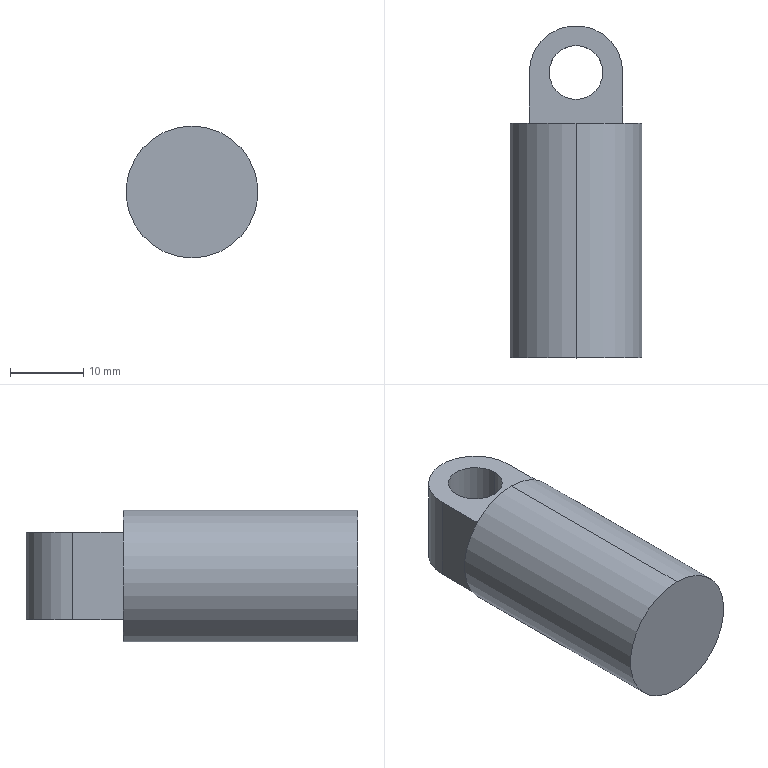Part | SolidWorks | features Cut 1, Extrusion 1, ICE 1 | 1 solid | 11 faces | box 18 x 45.316 x 18 mm | volume 9465 mm3 | plane 6 | cylinder 5 | commonest cylinder face diameters 7.349 x2 18 x2 12.778 x1
STEP:
#1=CARTESIAN_POINT('',(-30.863,-16.288,16.608));
#2=VERTEX_POINT('',#1);
#3=CARTESIAN_POINT('',(-23.514,-16.288,16.608));
#4=VERTEX_POINT('',#3);
#5=CARTESIAN_POINT('',(-27.189,-16.288,16.608));
#6=DIRECTION('',(0.,0.,1.));
#7=DIRECTION('',(-1.,0.,0.));
#8=AXIS2_PLACEMENT_3D('',#5,#6,#7);
#9=CIRCLE('',#8,3.675);
#10=EDGE_CURVE('',#2,#4,#9,.T.);
#11=ORIENTED_EDGE('',*,*,#10,.T.);
#12=CARTESIAN_POINT('',(-23.514,-16.288,4.608));
#13=VERTEX_POINT('',#12);
#14=CARTESIAN_POINT('',(-23.514,-16.288,27.001));
#15=DIRECTION('',(0.,0.,-1.));
#16=VECTOR('',#15,1000.);
#17=LINE('',#14,#16);
#18=EDGE_CURVE('',#4,#13,#17,.T.);
#19=ORIENTED_EDGE('',*,*,#18,.T.);
#20=CARTESIAN_POINT('',(-30.863,-16.288,4.608));
#21=VERTEX_POINT('',#20);
#22=CARTESIAN_POINT('',(-27.189,-16.288,4.608));
#23=DIRECTION('',(0.,0.,-1.));
#24=DIRECTION('',(-1.,0.,0.));
#25=AXIS2_PLACEMENT_3D('',#22,#23,#24);
#26=CIRCLE('',#25,3.675);
#27=EDGE_CURVE('',#13,#21,#26,.T.);
#28=ORIENTED_EDGE('',*,*,#27,.T.);
#29=CARTESIAN_POINT('',(-30.863,-16.288,27.001));
#30=DIRECTION('',(0.,0.,-1.));
#31=VECTOR('',#30,1000.);
#32=LINE('',#29,#31);
#33=EDGE_CURVE('',#2,#21,#32,.T.);
#34=ORIENTED_EDGE('',*,*,#33,.F.);
#35=EDGE_LOOP('',(#11,#19,#28,#34));
#36=FACE_OUTER_BOUND('',#35,.T.);
#37=CARTESIAN_POINT('',(-27.189,-16.288,27.001));
#38=DIRECTION('',(0.,0.,-1.));
#39=DIRECTION('',(-1.,0.,0.));
#40=AXIS2_PLACEMENT_3D('',#37,#38,#39);
#41=CYLINDRICAL_SURFACE('',#40,3.675);
#42=ADVANCED_FACE('',(#36),#41,.F.);
#43=CARTESIAN_POINT('',(-27.189,-55.215,1.608));
#44=VERTEX_POINT('',#43);
#45=CARTESIAN_POINT('',(-27.189,-55.215,19.608));
#46=VERTEX_POINT('',#45);
#47=CARTESIAN_POINT('',(-27.189,-55.215,10.608));
#48=DIRECTION('',(0.,-1.,0.));
#49=DIRECTION('',(0.,0.,-1.));
#50=AXIS2_PLACEMENT_3D('',#47,#48,#49);
#51=CIRCLE('',#50,9.);
#52=EDGE_CURVE('',#44,#46,#51,.T.);
#53=ORIENTED_EDGE('',*,*,#52,.F.);
#54=CARTESIAN_POINT('',(-27.189,-23.215,1.608));
#55=VERTEX_POINT('',#54);
#56=CARTESIAN_POINT('',(-27.189,-55.215,1.608));
#57=DIRECTION('',(0.,1.,0.));
#58=VECTOR('',#57,1000.);
#59=LINE('',#56,#58);
#60=EDGE_CURVE('',#44,#55,#59,.T.);
#61=ORIENTED_EDGE('',*,*,#60,.T.);
#62=CARTESIAN_POINT('',(-27.189,-23.215,19.608));
#63=VERTEX_POINT('',#62);
#64=CARTESIAN_POINT('',(-27.189,-23.215,10.608));
#65=DIRECTION('',(0.,-1.,0.));
#66=DIRECTION('',(0.,0.,-1.));
#67=AXIS2_PLACEMENT_3D('',#64,#65,#66);
#68=CIRCLE('',#67,9.);
#69=EDGE_CURVE('',#55,#63,#68,.T.);
#70=ORIENTED_EDGE('',*,*,#69,.T.);
#71=CARTESIAN_POINT('',(-27.189,-55.215,19.608));
#72=DIRECTION('',(0.,1.,0.));
#73=VECTOR('',#72,1000.);
#74=LINE('',#71,#73);
#75=EDGE_CURVE('',#46,#63,#74,.T.);
#76=ORIENTED_EDGE('',*,*,#75,.F.);
#77=EDGE_LOOP('',(#53,#61,#70,#76));
#78=FACE_OUTER_BOUND('',#77,.T.);
#79=CARTESIAN_POINT('',(-27.189,-55.215,10.608));
#80=DIRECTION('',(0.,1.,0.));
#81=DIRECTION('',(0.,0.,1.));
#82=AXIS2_PLACEMENT_3D('',#79,#80,#81);
#83=CYLINDRICAL_SURFACE('',#82,9.);
#84=ADVANCED_FACE('',(#78),#83,.T.);
#85=CARTESIAN_POINT('',(-33.578,-16.288,16.608));
#86=VERTEX_POINT('',#85);
#87=CARTESIAN_POINT('',(-20.8,-16.288,16.608));
#88=VERTEX_POINT('',#87);
#89=CARTESIAN_POINT('',(-27.189,-16.288,16.608));
#90=DIRECTION('',(0.,0.,-1.));
#91=DIRECTION('',(-1.,0.,0.));
#92=AXIS2_PLACEMENT_3D('',#89,#90,#91);
#93=CIRCLE('',#92,6.389);
#94=EDGE_CURVE('',#86,#88,#93,.T.);
#95=ORIENTED_EDGE('',*,*,#94,.T.);
#96=CARTESIAN_POINT('',(-20.8,-16.288,4.608));
#97=VERTEX_POINT('',#96);
#98=CARTESIAN_POINT('',(-20.8,-16.288,4.608));
#99=DIRECTION('',(0.,0.,1.));
#100=VECTOR('',#99,1000.);
#101=LINE('',#98,#100);
#102=EDGE_CURVE('',#97,#88,#101,.T.);
#103=ORIENTED_EDGE('',*,*,#102,.F.);
#104=CARTESIAN_POINT('',(-33.578,-16.288,4.608));
#105=VERTEX_POINT('',#104);
#106=CARTESIAN_POINT('',(-27.189,-16.288,4.608));
#107=DIRECTION('',(0.,0.,-1.));
#108=DIRECTION('',(-1.,0.,0.));
#109=AXIS2_PLACEMENT_3D('',#106,#107,#108);
#110=CIRCLE('',#109,6.389);
#111=EDGE_CURVE('',#105,#97,#110,.T.);
#112=ORIENTED_EDGE('',*,*,#111,.F.);
#113=CARTESIAN_POINT('',(-33.578,-16.288,4.608));
#114=DIRECTION('',(0.,0.,1.));
#115=VECTOR('',#114,1000.);
#116=LINE('',#113,#115);
#117=EDGE_CURVE('',#105,#86,#116,.T.);
#118=ORIENTED_EDGE('',*,*,#117,.T.);
#119=EDGE_LOOP('',(#95,#103,#112,#118));
#120=FACE_OUTER_BOUND('',#119,.T.);
#121=CARTESIAN_POINT('',(-27.189,-16.288,4.608));
#122=DIRECTION('',(0.,0.,1.));
#123=DIRECTION('',(1.,0.,0.));
#124=AXIS2_PLACEMENT_3D('',#121,#122,#123);
#125=CYLINDRICAL_SURFACE('',#124,6.389);
#126=ADVANCED_FACE('',(#120),#125,.T.);
#127=CARTESIAN_POINT('',(-20.8,-23.215,16.608));
#128=VERTEX_POINT('',#127);
#129=CARTESIAN_POINT('',(-20.8,-16.288,16.608));
#130=DIRECTION('',(0.,-1.,0.));
#131=VECTOR('',#130,1000.);
#132=LINE('',#129,#131);
#133=EDGE_CURVE('',#88,#128,#132,.T.);
#134=ORIENTED_EDGE('',*,*,#133,.T.);
#135=CARTESIAN_POINT('',(-20.8,-23.215,4.608));
#136=VERTEX_POINT('',#135);
#137=CARTESIAN_POINT('',(-20.8,-23.215,4.608));
#138=DIRECTION('',(0.,0.,1.));
#139=VECTOR('',#138,1000.);
#140=LINE('',#137,#139);
#141=EDGE_CURVE('',#136,#128,#140,.T.);
#142=ORIENTED_EDGE('',*,*,#141,.F.);
#143=CARTESIAN_POINT('',(-20.8,-16.288,4.608));
#144=DIRECTION('',(0.,-1.,0.));
#145=VECTOR('',#144,1000.);
#146=LINE('',#143,#145);
#147=EDGE_CURVE('',#97,#136,#146,.T.);
#148=ORIENTED_EDGE('',*,*,#147,.F.);
#149=ORIENTED_EDGE('',*,*,#102,.T.);
#150=EDGE_LOOP('',(#134,#142,#148,#149));
#151=FACE_OUTER_BOUND('',#150,.T.);
#152=CARTESIAN_POINT('',(-20.8,-16.288,4.608));
#153=DIRECTION('',(-1.,0.,0.));
#154=DIRECTION('',(0.,0.,1.));
#155=AXIS2_PLACEMENT_3D('',#152,#153,#154);
#156=PLANE('',#155);
#157=ADVANCED_FACE('',(#151),#156,.F.);
#158=CARTESIAN_POINT('',(-33.578,-23.215,16.608));
#159=VERTEX_POINT('',#158);
#160=CARTESIAN_POINT('',(-33.578,-23.215,16.608));
#161=DIRECTION('',(0.,1.,0.));
#162=VECTOR('',#161,1000.);
#163=LINE('',#160,#162);
#164=EDGE_CURVE('',#159,#86,#163,.T.);
#165=ORIENTED_EDGE('',*,*,#164,.T.);
#166=ORIENTED_EDGE('',*,*,#117,.F.);
#167=CARTESIAN_POINT('',(-33.578,-23.215,4.608));
#168=VERTEX_POINT('',#167);
#169=CARTESIAN_POINT('',(-33.578,-23.215,4.608));
#170=DIRECTION('',(0.,1.,0.));
#171=VECTOR('',#170,1000.);
#172=LINE('',#169,#171);
#173=EDGE_CURVE('',#168,#105,#172,.T.);
#174=ORIENTED_EDGE('',*,*,#173,.F.);
#175=CARTESIAN_POINT('',(-33.578,-23.215,4.608));
#176=DIRECTION('',(0.,0.,1.));
#177=VECTOR('',#176,1000.);
#178=LINE('',#175,#177);
#179=EDGE_CURVE('',#168,#159,#178,.T.);
#180=ORIENTED_EDGE('',*,*,#179,.T.);
#181=EDGE_LOOP('',(#165,#166,#174,#180));
#182=FACE_OUTER_BOUND('',#181,.T.);
#183=CARTESIAN_POINT('',(-33.578,-23.215,4.608));
#184=DIRECTION('',(1.,0.,0.));
#185=DIRECTION('',(0.,0.,-1.));
#186=AXIS2_PLACEMENT_3D('',#183,#184,#185);
#187=PLANE('',#186);
#188=ADVANCED_FACE('',(#182),#187,.F.);
#189=CARTESIAN_POINT('',(-27.189,-16.288,4.608));
#190=DIRECTION('',(0.,0.,-1.));
#191=DIRECTION('',(-1.,0.,0.));
#192=AXIS2_PLACEMENT_3D('',#189,#190,#191);
#193=CIRCLE('',#192,3.675);
#194=EDGE_CURVE('',#21,#13,#193,.T.);
#195=ORIENTED_EDGE('',*,*,#194,.F.);
#196=ORIENTED_EDGE('',*,*,#27,.F.);
#197=EDGE_LOOP('',(#195,#196));
#198=FACE_BOUND('',#197,.T.);
#199=ORIENTED_EDGE('',*,*,#111,.T.);
#200=ORIENTED_EDGE('',*,*,#147,.T.);
#201=CARTESIAN_POINT('',(-20.8,-23.215,4.608));
#202=DIRECTION('',(-1.,0.,0.));
#203=VECTOR('',#202,1000.);
#204=LINE('',#201,#203);
#205=EDGE_CURVE('',#136,#168,#204,.T.);
#206=ORIENTED_EDGE('',*,*,#205,.T.);
#207=ORIENTED_EDGE('',*,*,#173,.T.);
#208=EDGE_LOOP('',(#199,#200,#206,#207));
#209=FACE_OUTER_BOUND('',#208,.T.);
#210=CARTESIAN_POINT('',(-27.189,-16.288,4.608));
#211=DIRECTION('',(0.,0.,-1.));
#212=DIRECTION('',(-1.,0.,0.));
#213=AXIS2_PLACEMENT_3D('',#210,#211,#212);
#214=PLANE('',#213);
#215=ADVANCED_FACE('',(#198,#209),#214,.T.);
#216=ORIENTED_EDGE('',*,*,#10,.F.);
#217=CARTESIAN_POINT('',(-27.189,-16.288,16.608));
#218=DIRECTION('',(0.,0.,1.));
#219=DIRECTION('',(-1.,0.,0.));
#220=AXIS2_PLACEMENT_3D('',#217,#218,#219);
#221=CIRCLE('',#220,3.675);
#222=EDGE_CURVE('',#4,#2,#221,.T.);
#223=ORIENTED_EDGE('',*,*,#222,.F.);
#224=EDGE_LOOP('',(#216,#223));
#225=FACE_BOUND('',#224,.T.);
#226=ORIENTED_EDGE('',*,*,#94,.F.);
#227=ORIENTED_EDGE('',*,*,#164,.F.);
#228=CARTESIAN_POINT('',(-20.8,-23.215,16.608));
#229=DIRECTION('',(-1.,0.,0.));
#230=VECTOR('',#229,1000.);
#231=LINE('',#228,#230);
#232=EDGE_CURVE('',#128,#159,#231,.T.);
#233=ORIENTED_EDGE('',*,*,#232,.F.);
#234=ORIENTED_EDGE('',*,*,#133,.F.);
#235=EDGE_LOOP('',(#226,#227,#233,#234));
#236=FACE_OUTER_BOUND('',#235,.T.);
#237=CARTESIAN_POINT('',(-27.189,-16.288,16.608));
#238=DIRECTION('',(0.,0.,-1.));
#239=DIRECTION('',(-1.,0.,0.));
#240=AXIS2_PLACEMENT_3D('',#237,#238,#239);
#241=PLANE('',#240);
#242=ADVANCED_FACE('',(#225,#236),#241,.F.);
#243=CARTESIAN_POINT('',(-27.189,-23.215,10.608));
#244=DIRECTION('',(0.,-1.,0.));
#245=DIRECTION('',(0.,0.,-1.));
#246=AXIS2_PLACEMENT_3D('',#243,#244,#245);
#247=CIRCLE('',#246,9.);
#248=EDGE_CURVE('',#63,#55,#247,.T.);
#249=ORIENTED_EDGE('',*,*,#248,.F.);
#250=ORIENTED_EDGE('',*,*,#69,.F.);
#251=EDGE_LOOP('',(#249,#250));
#252=FACE_OUTER_BOUND('',#251,.T.);
#253=ORIENTED_EDGE('',*,*,#141,.T.);
#254=ORIENTED_EDGE('',*,*,#232,.T.);
#255=ORIENTED_EDGE('',*,*,#179,.F.);
#256=ORIENTED_EDGE('',*,*,#205,.F.);
#257=EDGE_LOOP('',(#253,#254,#255,#256));
#258=FACE_BOUND('',#257,.T.);
#259=CARTESIAN_POINT('',(-27.189,-23.215,10.608));
#260=DIRECTION('',(0.,-1.,0.));
#261=DIRECTION('',(0.,0.,-1.));
#262=AXIS2_PLACEMENT_3D('',#259,#260,#261);
#263=PLANE('',#262);
#264=ADVANCED_FACE('',(#252,#258),#263,.F.);
#265=ORIENTED_EDGE('',*,*,#60,.F.);
#266=CARTESIAN_POINT('',(-27.189,-55.215,10.608));
#267=DIRECTION('',(0.,-1.,0.));
#268=DIRECTION('',(0.,0.,-1.));
#269=AXIS2_PLACEMENT_3D('',#266,#267,#268);
#270=CIRCLE('',#269,9.);
#271=EDGE_CURVE('',#46,#44,#270,.T.);
#272=ORIENTED_EDGE('',*,*,#271,.F.);
#273=ORIENTED_EDGE('',*,*,#75,.T.);
#274=ORIENTED_EDGE('',*,*,#248,.T.);
#275=EDGE_LOOP('',(#265,#272,#273,#274));
#276=FACE_OUTER_BOUND('',#275,.T.);
#277=CARTESIAN_POINT('',(-27.189,-55.215,10.608));
#278=DIRECTION('',(0.,1.,0.));
#279=DIRECTION('',(0.,0.,1.));
#280=AXIS2_PLACEMENT_3D('',#277,#278,#279);
#281=CYLINDRICAL_SURFACE('',#280,9.);
#282=ADVANCED_FACE('',(#276),#281,.T.);
#283=ORIENTED_EDGE('',*,*,#271,.T.);
#284=ORIENTED_EDGE('',*,*,#52,.T.);
#285=EDGE_LOOP('',(#283,#284));
#286=FACE_OUTER_BOUND('',#285,.T.);
#287=CARTESIAN_POINT('',(-27.189,-55.215,10.608));
#288=DIRECTION('',(0.,-1.,0.));
#289=DIRECTION('',(0.,0.,-1.));
#290=AXIS2_PLACEMENT_3D('',#287,#288,#289);
#291=PLANE('',#290);
#292=ADVANCED_FACE('',(#286),#291,.T.);
#293=ORIENTED_EDGE('',*,*,#18,.F.);
#294=ORIENTED_EDGE('',*,*,#222,.T.);
#295=ORIENTED_EDGE('',*,*,#33,.T.);
#296=ORIENTED_EDGE('',*,*,#194,.T.);
#297=EDGE_LOOP('',(#293,#294,#295,#296));
#298=FACE_OUTER_BOUND('',#297,.T.);
#299=CARTESIAN_POINT('',(-27.189,-16.288,27.001));
#300=DIRECTION('',(0.,0.,-1.));
#301=DIRECTION('',(-1.,0.,0.));
#302=AXIS2_PLACEMENT_3D('',#299,#300,#301);
#303=CYLINDRICAL_SURFACE('',#302,3.675);
#304=ADVANCED_FACE('',(#298),#303,.F.);
#305=CLOSED_SHELL('',(#42,#84,#126,#157,#188,#215,#242,#264,#282,#292,#304));
#306=MANIFOLD_SOLID_BREP('',#305);
#307=CARTESIAN_POINT('',(0.,0.,0.));
#308=DIRECTION('',(0.,0.,1.));
#309=DIRECTION('',(1.,0.,0.));
#310=AXIS2_PLACEMENT_3D('',#307,#308,#309);
#311=(LENGTH_UNIT()NAMED_UNIT(*)SI_UNIT(.MILLI.,.METRE.));
#312=UNCERTAINTY_MEASURE_WITH_UNIT(LENGTH_MEASURE(0.00001),#311,'','');
#313=(NAMED_UNIT(*)PLANE_ANGLE_UNIT()SI_UNIT($,.RADIAN.));
#314=(NAMED_UNIT(*)SI_UNIT($,.STERADIAN.)SOLID_ANGLE_UNIT());
#315=(GEOMETRIC_REPRESENTATION_CONTEXT(3)GLOBAL_UNCERTAINTY_ASSIGNED_CONTEXT((#312))GLOBAL_UNIT_ASSIGNED_CONTEXT((#311,#313,#314))REPRESENTATION_CONTEXT('',''));
#316=ADVANCED_BREP_SHAPE_REPRESENTATION('',(#306,#310),#315);